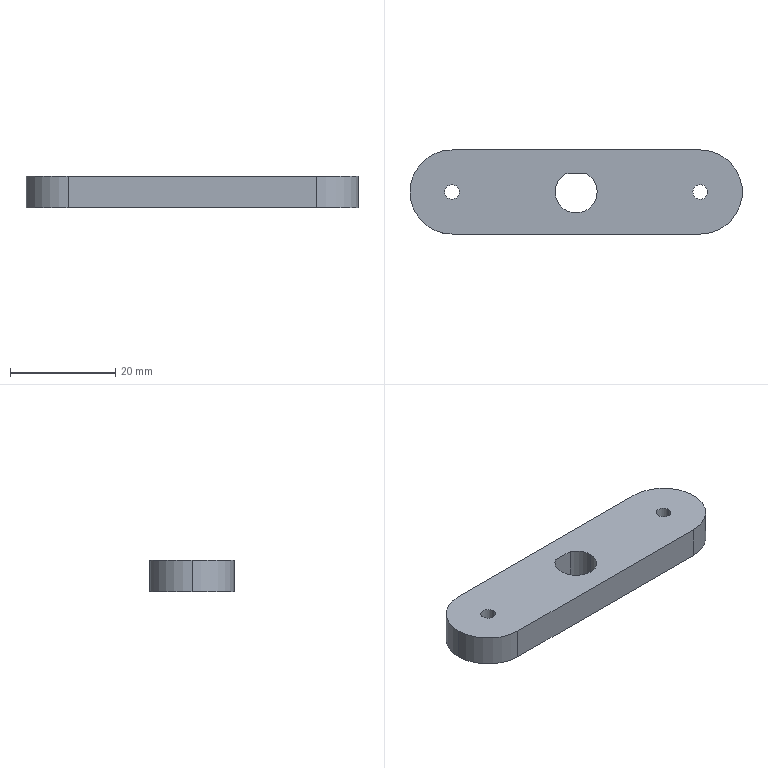Part | SolidWorks | features ICE 3, Extrusion 1 | 1 solid | 18 faces | box 63.2 x 16 x 6 mm | volume 5359 mm3 | cylinder 12 | plane 6 | commonest cylinder face diameters 2.8 x4 8 x3 16 x3 2 x2
STEP:
#1=CARTESIAN_POINT('',(-1.,4.5,3.));
#2=VERTEX_POINT('',#1);
#3=CARTESIAN_POINT('',(1.,4.5,3.));
#4=VERTEX_POINT('',#3);
#5=CARTESIAN_POINT('',(0.,4.5,3.));
#6=DIRECTION('',(0.,-1.,0.));
#7=DIRECTION('',(0.,0.,1.));
#8=AXIS2_PLACEMENT_3D('',#5,#6,#7);
#9=CIRCLE('',#8,1.);
#10=EDGE_CURVE('',#2,#4,#9,.T.);
#11=ORIENTED_EDGE('',*,*,#10,.T.);
#12=CARTESIAN_POINT('',(1.,8.,3.));
#13=VERTEX_POINT('',#12);
#14=CARTESIAN_POINT('',(1.,3.,3.));
#15=DIRECTION('',(0.,1.,0.));
#16=VECTOR('',#15,1000.);
#17=LINE('',#14,#16);
#18=EDGE_CURVE('',#4,#13,#17,.T.);
#19=ORIENTED_EDGE('',*,*,#18,.T.);
#20=CARTESIAN_POINT('',(-1.,8.,3.));
#21=VERTEX_POINT('',#20);
#22=CARTESIAN_POINT('',(0.,8.,3.));
#23=DIRECTION('',(0.,1.,0.));
#24=DIRECTION('',(-1.,0.,0.));
#25=AXIS2_PLACEMENT_3D('',#22,#23,#24);
#26=CIRCLE('',#25,1.);
#27=EDGE_CURVE('',#13,#21,#26,.T.);
#28=ORIENTED_EDGE('',*,*,#27,.T.);
#29=CARTESIAN_POINT('',(-1.,3.,3.));
#30=DIRECTION('',(0.,1.,0.));
#31=VECTOR('',#30,1000.);
#32=LINE('',#29,#31);
#33=EDGE_CURVE('',#2,#21,#32,.T.);
#34=ORIENTED_EDGE('',*,*,#33,.F.);
#35=EDGE_LOOP('',(#11,#19,#28,#34));
#36=FACE_OUTER_BOUND('',#35,.T.);
#37=CARTESIAN_POINT('',(0.,3.,3.));
#38=DIRECTION('',(0.,1.,0.));
#39=DIRECTION('',(-1.,0.,0.));
#40=AXIS2_PLACEMENT_3D('',#37,#38,#39);
#41=CYLINDRICAL_SURFACE('',#40,1.);
#42=ADVANCED_FACE('',(#36),#41,.F.);
#43=CARTESIAN_POINT('',(-25.,0.,0.));
#44=VERTEX_POINT('',#43);
#45=CARTESIAN_POINT('',(-22.2,0.,0.));
#46=VERTEX_POINT('',#45);
#47=CARTESIAN_POINT('',(-23.6,0.,0.));
#48=DIRECTION('',(0.,0.,1.));
#49=DIRECTION('',(1.,0.,0.));
#50=AXIS2_PLACEMENT_3D('',#47,#48,#49);
#51=CIRCLE('',#50,1.4);
#52=EDGE_CURVE('',#44,#46,#51,.T.);
#53=ORIENTED_EDGE('',*,*,#52,.F.);
#54=CARTESIAN_POINT('',(-25.,0.,6.));
#55=VERTEX_POINT('',#54);
#56=CARTESIAN_POINT('',(-25.,0.,0.));
#57=DIRECTION('',(0.,0.,1.));
#58=VECTOR('',#57,1000.);
#59=LINE('',#56,#58);
#60=EDGE_CURVE('',#44,#55,#59,.T.);
#61=ORIENTED_EDGE('',*,*,#60,.T.);
#62=CARTESIAN_POINT('',(-22.2,0.,6.));
#63=VERTEX_POINT('',#62);
#64=CARTESIAN_POINT('',(-23.6,0.,6.));
#65=DIRECTION('',(0.,0.,1.));
#66=DIRECTION('',(1.,0.,0.));
#67=AXIS2_PLACEMENT_3D('',#64,#65,#66);
#68=CIRCLE('',#67,1.4);
#69=EDGE_CURVE('',#55,#63,#68,.T.);
#70=ORIENTED_EDGE('',*,*,#69,.T.);
#71=CARTESIAN_POINT('',(-22.2,0.,0.));
#72=DIRECTION('',(0.,0.,1.));
#73=VECTOR('',#72,1000.);
#74=LINE('',#71,#73);
#75=EDGE_CURVE('',#46,#63,#74,.T.);
#76=ORIENTED_EDGE('',*,*,#75,.F.);
#77=EDGE_LOOP('',(#53,#61,#70,#76));
#78=FACE_OUTER_BOUND('',#77,.T.);
#79=CARTESIAN_POINT('',(-23.6,0.,0.));
#80=DIRECTION('',(0.,0.,1.));
#81=DIRECTION('',(1.,0.,0.));
#82=AXIS2_PLACEMENT_3D('',#79,#80,#81);
#83=CYLINDRICAL_SURFACE('',#82,1.4);
#84=ADVANCED_FACE('',(#78),#83,.F.);
#85=CARTESIAN_POINT('',(22.2,0.,0.));
#86=VERTEX_POINT('',#85);
#87=CARTESIAN_POINT('',(25.,0.,0.));
#88=VERTEX_POINT('',#87);
#89=CARTESIAN_POINT('',(23.6,0.,0.));
#90=DIRECTION('',(0.,0.,1.));
#91=DIRECTION('',(1.,0.,0.));
#92=AXIS2_PLACEMENT_3D('',#89,#90,#91);
#93=CIRCLE('',#92,1.4);
#94=EDGE_CURVE('',#86,#88,#93,.T.);
#95=ORIENTED_EDGE('',*,*,#94,.F.);
#96=CARTESIAN_POINT('',(22.2,0.,6.));
#97=VERTEX_POINT('',#96);
#98=CARTESIAN_POINT('',(22.2,0.,0.));
#99=DIRECTION('',(0.,0.,1.));
#100=VECTOR('',#99,1000.);
#101=LINE('',#98,#100);
#102=EDGE_CURVE('',#86,#97,#101,.T.);
#103=ORIENTED_EDGE('',*,*,#102,.T.);
#104=CARTESIAN_POINT('',(25.,0.,6.));
#105=VERTEX_POINT('',#104);
#106=CARTESIAN_POINT('',(23.6,0.,6.));
#107=DIRECTION('',(0.,0.,1.));
#108=DIRECTION('',(1.,0.,0.));
#109=AXIS2_PLACEMENT_3D('',#106,#107,#108);
#110=CIRCLE('',#109,1.4);
#111=EDGE_CURVE('',#97,#105,#110,.T.);
#112=ORIENTED_EDGE('',*,*,#111,.T.);
#113=CARTESIAN_POINT('',(25.,0.,0.));
#114=DIRECTION('',(0.,0.,1.));
#115=VECTOR('',#114,1000.);
#116=LINE('',#113,#115);
#117=EDGE_CURVE('',#88,#105,#116,.T.);
#118=ORIENTED_EDGE('',*,*,#117,.F.);
#119=EDGE_LOOP('',(#95,#103,#112,#118));
#120=FACE_OUTER_BOUND('',#119,.T.);
#121=CARTESIAN_POINT('',(23.6,0.,0.));
#122=DIRECTION('',(0.,0.,1.));
#123=DIRECTION('',(1.,0.,0.));
#124=AXIS2_PLACEMENT_3D('',#121,#122,#123);
#125=CYLINDRICAL_SURFACE('',#124,1.4);
#126=ADVANCED_FACE('',(#120),#125,.F.);
#127=CARTESIAN_POINT('',(-4.,0.,6.));
#128=VERTEX_POINT('',#127);
#129=CARTESIAN_POINT('',(4.,0.,6.));
#130=VERTEX_POINT('',#129);
#131=CARTESIAN_POINT('',(0.,0.,6.));
#132=DIRECTION('',(0.,0.,1.));
#133=DIRECTION('',(1.,0.,0.));
#134=AXIS2_PLACEMENT_3D('',#131,#132,#133);
#135=CIRCLE('',#134,4.);
#136=EDGE_CURVE('',#128,#130,#135,.T.);
#137=ORIENTED_EDGE('',*,*,#136,.T.);
#138=CARTESIAN_POINT('',(4.,0.,0.));
#139=VERTEX_POINT('',#138);
#140=CARTESIAN_POINT('',(4.,0.,6.));
#141=DIRECTION('',(0.,0.,-1.));
#142=VECTOR('',#141,1000.);
#143=LINE('',#140,#142);
#144=EDGE_CURVE('',#130,#139,#143,.T.);
#145=ORIENTED_EDGE('',*,*,#144,.T.);
#146=CARTESIAN_POINT('',(-4.,0.,0.));
#147=VERTEX_POINT('',#146);
#148=CARTESIAN_POINT('',(0.,0.,0.));
#149=DIRECTION('',(0.,0.,1.));
#150=DIRECTION('',(1.,0.,0.));
#151=AXIS2_PLACEMENT_3D('',#148,#149,#150);
#152=CIRCLE('',#151,4.);
#153=EDGE_CURVE('',#147,#139,#152,.T.);
#154=ORIENTED_EDGE('',*,*,#153,.F.);
#155=CARTESIAN_POINT('',(-4.,0.,6.));
#156=DIRECTION('',(0.,0.,-1.));
#157=VECTOR('',#156,1000.);
#158=LINE('',#155,#157);
#159=EDGE_CURVE('',#128,#147,#158,.T.);
#160=ORIENTED_EDGE('',*,*,#159,.F.);
#161=EDGE_LOOP('',(#137,#145,#154,#160));
#162=FACE_OUTER_BOUND('',#161,.T.);
#163=CARTESIAN_POINT('',(0.,0.,6.));
#164=DIRECTION('',(0.,0.,-1.));
#165=DIRECTION('',(-1.,0.,0.));
#166=AXIS2_PLACEMENT_3D('',#163,#164,#165);
#167=CYLINDRICAL_SURFACE('',#166,4.);
#168=ADVANCED_FACE('',(#162),#167,.F.);
#169=CARTESIAN_POINT('',(-1.936,3.5,6.));
#170=VERTEX_POINT('',#169);
#171=CARTESIAN_POINT('',(0.,0.,6.));
#172=DIRECTION('',(0.,0.,1.));
#173=DIRECTION('',(1.,0.,0.));
#174=AXIS2_PLACEMENT_3D('',#171,#172,#173);
#175=CIRCLE('',#174,4.);
#176=EDGE_CURVE('',#170,#128,#175,.T.);
#177=ORIENTED_EDGE('',*,*,#176,.T.);
#178=ORIENTED_EDGE('',*,*,#159,.T.);
#179=CARTESIAN_POINT('',(-1.936,3.5,0.));
#180=VERTEX_POINT('',#179);
#181=CARTESIAN_POINT('',(0.,0.,0.));
#182=DIRECTION('',(0.,0.,1.));
#183=DIRECTION('',(1.,0.,0.));
#184=AXIS2_PLACEMENT_3D('',#181,#182,#183);
#185=CIRCLE('',#184,4.);
#186=EDGE_CURVE('',#180,#147,#185,.T.);
#187=ORIENTED_EDGE('',*,*,#186,.F.);
#188=CARTESIAN_POINT('',(-1.936,3.5,6.));
#189=DIRECTION('',(0.,0.,-1.));
#190=VECTOR('',#189,1000.);
#191=LINE('',#188,#190);
#192=EDGE_CURVE('',#170,#180,#191,.T.);
#193=ORIENTED_EDGE('',*,*,#192,.F.);
#194=EDGE_LOOP('',(#177,#178,#187,#193));
#195=FACE_OUTER_BOUND('',#194,.T.);
#196=CARTESIAN_POINT('',(0.,0.,6.));
#197=DIRECTION('',(0.,0.,-1.));
#198=DIRECTION('',(-1.,0.,0.));
#199=AXIS2_PLACEMENT_3D('',#196,#197,#198);
#200=CYLINDRICAL_SURFACE('',#199,4.);
#201=ADVANCED_FACE('',(#195),#200,.F.);
#202=CARTESIAN_POINT('',(-31.6,0.,6.));
#203=VERTEX_POINT('',#202);
#204=CARTESIAN_POINT('',(-23.6,-8.,6.));
#205=VERTEX_POINT('',#204);
#206=CARTESIAN_POINT('',(-23.6,0.,6.));
#207=DIRECTION('',(0.,0.,1.));
#208=DIRECTION('',(1.,0.,0.));
#209=AXIS2_PLACEMENT_3D('',#206,#207,#208);
#210=CIRCLE('',#209,8.);
#211=EDGE_CURVE('',#203,#205,#210,.T.);
#212=ORIENTED_EDGE('',*,*,#211,.F.);
#213=CARTESIAN_POINT('',(-31.6,0.,0.));
#214=VERTEX_POINT('',#213);
#215=CARTESIAN_POINT('',(-31.6,0.,6.));
#216=DIRECTION('',(0.,0.,-1.));
#217=VECTOR('',#216,1000.);
#218=LINE('',#215,#217);
#219=EDGE_CURVE('',#203,#214,#218,.T.);
#220=ORIENTED_EDGE('',*,*,#219,.T.);
#221=CARTESIAN_POINT('',(-23.6,-8.,0.));
#222=VERTEX_POINT('',#221);
#223=CARTESIAN_POINT('',(-23.6,0.,0.));
#224=DIRECTION('',(0.,0.,1.));
#225=DIRECTION('',(1.,0.,0.));
#226=AXIS2_PLACEMENT_3D('',#223,#224,#225);
#227=CIRCLE('',#226,8.);
#228=EDGE_CURVE('',#214,#222,#227,.T.);
#229=ORIENTED_EDGE('',*,*,#228,.T.);
#230=CARTESIAN_POINT('',(-23.6,-8.,6.));
#231=DIRECTION('',(0.,0.,-1.));
#232=VECTOR('',#231,1000.);
#233=LINE('',#230,#232);
#234=EDGE_CURVE('',#205,#222,#233,.T.);
#235=ORIENTED_EDGE('',*,*,#234,.F.);
#236=EDGE_LOOP('',(#212,#220,#229,#235));
#237=FACE_OUTER_BOUND('',#236,.T.);
#238=CARTESIAN_POINT('',(-23.6,0.,6.));
#239=DIRECTION('',(0.,0.,-1.));
#240=DIRECTION('',(-1.,0.,0.));
#241=AXIS2_PLACEMENT_3D('',#238,#239,#240);
#242=CYLINDRICAL_SURFACE('',#241,8.);
#243=ADVANCED_FACE('',(#237),#242,.T.);
#244=ORIENTED_EDGE('',*,*,#176,.F.);
#245=CARTESIAN_POINT('',(1.936,3.5,6.));
#246=VERTEX_POINT('',#245);
#247=CARTESIAN_POINT('',(2.48,3.5,6.));
#248=DIRECTION('',(-1.,0.,0.));
#249=VECTOR('',#248,1000.);
#250=LINE('',#247,#249);
#251=EDGE_CURVE('',#246,#170,#250,.T.);
#252=ORIENTED_EDGE('',*,*,#251,.F.);
#253=CARTESIAN_POINT('',(0.,0.,6.));
#254=DIRECTION('',(0.,0.,1.));
#255=DIRECTION('',(1.,0.,0.));
#256=AXIS2_PLACEMENT_3D('',#253,#254,#255);
#257=CIRCLE('',#256,4.);
#258=EDGE_CURVE('',#130,#246,#257,.T.);
#259=ORIENTED_EDGE('',*,*,#258,.F.);
#260=ORIENTED_EDGE('',*,*,#136,.F.);
#261=EDGE_LOOP('',(#244,#252,#259,#260));
#262=FACE_BOUND('',#261,.T.);
#263=CARTESIAN_POINT('',(-23.6,0.,6.));
#264=DIRECTION('',(0.,0.,1.));
#265=DIRECTION('',(1.,0.,0.));
#266=AXIS2_PLACEMENT_3D('',#263,#264,#265);
#267=CIRCLE('',#266,1.4);
#268=EDGE_CURVE('',#63,#55,#267,.T.);
#269=ORIENTED_EDGE('',*,*,#268,.F.);
#270=ORIENTED_EDGE('',*,*,#69,.F.);
#271=EDGE_LOOP('',(#269,#270));
#272=FACE_BOUND('',#271,.T.);
#273=CARTESIAN_POINT('',(23.6,0.,6.));
#274=DIRECTION('',(0.,0.,1.));
#275=DIRECTION('',(1.,0.,0.));
#276=AXIS2_PLACEMENT_3D('',#273,#274,#275);
#277=CIRCLE('',#276,1.4);
#278=EDGE_CURVE('',#105,#97,#277,.T.);
#279=ORIENTED_EDGE('',*,*,#278,.F.);
#280=ORIENTED_EDGE('',*,*,#111,.F.);
#281=EDGE_LOOP('',(#279,#280));
#282=FACE_BOUND('',#281,.T.);
#283=CARTESIAN_POINT('',(-23.6,8.,6.));
#284=VERTEX_POINT('',#283);
#285=CARTESIAN_POINT('',(-23.6,0.,6.));
#286=DIRECTION('',(0.,0.,1.));
#287=DIRECTION('',(1.,0.,0.));
#288=AXIS2_PLACEMENT_3D('',#285,#286,#287);
#289=CIRCLE('',#288,8.);
#290=EDGE_CURVE('',#284,#203,#289,.T.);
#291=ORIENTED_EDGE('',*,*,#290,.T.);
#292=ORIENTED_EDGE('',*,*,#211,.T.);
#293=CARTESIAN_POINT('',(23.6,-8.,6.));
#294=VERTEX_POINT('',#293);
#295=CARTESIAN_POINT('',(-23.6,-8.,6.));
#296=DIRECTION('',(1.,0.,0.));
#297=VECTOR('',#296,1000.);
#298=LINE('',#295,#297);
#299=EDGE_CURVE('',#205,#294,#298,.T.);
#300=ORIENTED_EDGE('',*,*,#299,.T.);
#301=CARTESIAN_POINT('',(23.6,8.,6.));
#302=VERTEX_POINT('',#301);
#303=CARTESIAN_POINT('',(23.6,0.,6.));
#304=DIRECTION('',(0.,0.,1.));
#305=DIRECTION('',(1.,0.,0.));
#306=AXIS2_PLACEMENT_3D('',#303,#304,#305);
#307=CIRCLE('',#306,8.);
#308=EDGE_CURVE('',#294,#302,#307,.T.);
#309=ORIENTED_EDGE('',*,*,#308,.T.);
#310=CARTESIAN_POINT('',(-23.6,8.,6.));
#311=DIRECTION('',(-1.,0.,0.));
#312=VECTOR('',#311,1000.);
#313=LINE('',#310,#312);
#314=EDGE_CURVE('',#302,#284,#313,.T.);
#315=ORIENTED_EDGE('',*,*,#314,.T.);
#316=EDGE_LOOP('',(#291,#292,#300,#309,#315));
#317=FACE_OUTER_BOUND('',#316,.T.);
#318=CARTESIAN_POINT('',(-23.6,0.,6.));
#319=DIRECTION('',(0.,0.,1.));
#320=DIRECTION('',(1.,0.,0.));
#321=AXIS2_PLACEMENT_3D('',#318,#319,#320);
#322=PLANE('',#321);
#323=ADVANCED_FACE('',(#262,#272,#282,#317),#322,.T.);
#324=CARTESIAN_POINT('',(1.936,3.5,0.));
#325=VERTEX_POINT('',#324);
#326=CARTESIAN_POINT('',(2.48,3.5,0.));
#327=DIRECTION('',(-1.,0.,0.));
#328=VECTOR('',#327,1000.);
#329=LINE('',#326,#328);
#330=EDGE_CURVE('',#325,#180,#329,.T.);
#331=ORIENTED_EDGE('',*,*,#330,.T.);
#332=ORIENTED_EDGE('',*,*,#186,.T.);
#333=ORIENTED_EDGE('',*,*,#153,.T.);
#334=CARTESIAN_POINT('',(0.,0.,0.));
#335=DIRECTION('',(0.,0.,1.));
#336=DIRECTION('',(1.,0.,0.));
#337=AXIS2_PLACEMENT_3D('',#334,#335,#336);
#338=CIRCLE('',#337,4.);
#339=EDGE_CURVE('',#139,#325,#338,.T.);
#340=ORIENTED_EDGE('',*,*,#339,.T.);
#341=EDGE_LOOP('',(#331,#332,#333,#340));
#342=FACE_BOUND('',#341,.T.);
#343=CARTESIAN_POINT('',(-23.6,0.,0.));
#344=DIRECTION('',(0.,0.,1.));
#345=DIRECTION('',(1.,0.,0.));
#346=AXIS2_PLACEMENT_3D('',#343,#344,#345);
#347=CIRCLE('',#346,1.4);
#348=EDGE_CURVE('',#46,#44,#347,.T.);
#349=ORIENTED_EDGE('',*,*,#348,.T.);
#350=ORIENTED_EDGE('',*,*,#52,.T.);
#351=EDGE_LOOP('',(#349,#350));
#352=FACE_BOUND('',#351,.T.);
#353=CARTESIAN_POINT('',(23.6,0.,0.));
#354=DIRECTION('',(0.,0.,1.));
#355=DIRECTION('',(1.,0.,0.));
#356=AXIS2_PLACEMENT_3D('',#353,#354,#355);
#357=CIRCLE('',#356,1.4);
#358=EDGE_CURVE('',#88,#86,#357,.T.);
#359=ORIENTED_EDGE('',*,*,#358,.T.);
#360=ORIENTED_EDGE('',*,*,#94,.T.);
#361=EDGE_LOOP('',(#359,#360));
#362=FACE_BOUND('',#361,.T.);
#363=CARTESIAN_POINT('',(-23.6,8.,0.));
#364=VERTEX_POINT('',#363);
#365=CARTESIAN_POINT('',(-23.6,0.,0.));
#366=DIRECTION('',(0.,0.,1.));
#367=DIRECTION('',(1.,0.,0.));
#368=AXIS2_PLACEMENT_3D('',#365,#366,#367);
#369=CIRCLE('',#368,8.);
#370=EDGE_CURVE('',#364,#214,#369,.T.);
#371=ORIENTED_EDGE('',*,*,#370,.F.);
#372=CARTESIAN_POINT('',(23.6,8.,0.));
#373=VERTEX_POINT('',#372);
#374=CARTESIAN_POINT('',(-23.6,8.,0.));
#375=DIRECTION('',(-1.,0.,0.));
#376=VECTOR('',#375,1000.);
#377=LINE('',#374,#376);
#378=EDGE_CURVE('',#373,#364,#377,.T.);
#379=ORIENTED_EDGE('',*,*,#378,.F.);
#380=CARTESIAN_POINT('',(23.6,-8.,0.));
#381=VERTEX_POINT('',#380);
#382=CARTESIAN_POINT('',(23.6,0.,0.));
#383=DIRECTION('',(0.,0.,1.));
#384=DIRECTION('',(1.,0.,0.));
#385=AXIS2_PLACEMENT_3D('',#382,#383,#384);
#386=CIRCLE('',#385,8.);
#387=EDGE_CURVE('',#381,#373,#386,.T.);
#388=ORIENTED_EDGE('',*,*,#387,.F.);
#389=CARTESIAN_POINT('',(-23.6,-8.,0.));
#390=DIRECTION('',(1.,0.,0.));
#391=VECTOR('',#390,1000.);
#392=LINE('',#389,#391);
#393=EDGE_CURVE('',#222,#381,#392,.T.);
#394=ORIENTED_EDGE('',*,*,#393,.F.);
#395=ORIENTED_EDGE('',*,*,#228,.F.);
#396=EDGE_LOOP('',(#371,#379,#388,#394,#395));
#397=FACE_OUTER_BOUND('',#396,.T.);
#398=CARTESIAN_POINT('',(-23.6,0.,0.));
#399=DIRECTION('',(0.,0.,1.));
#400=DIRECTION('',(1.,0.,0.));
#401=AXIS2_PLACEMENT_3D('',#398,#399,#400);
#402=PLANE('',#401);
#403=ADVANCED_FACE('',(#342,#352,#362,#397),#402,.F.);
#404=ORIENTED_EDGE('',*,*,#219,.F.);
#405=ORIENTED_EDGE('',*,*,#290,.F.);
#406=CARTESIAN_POINT('',(-23.6,8.,6.));
#407=DIRECTION('',(0.,0.,-1.));
#408=VECTOR('',#407,1000.);
#409=LINE('',#406,#408);
#410=EDGE_CURVE('',#284,#364,#409,.T.);
#411=ORIENTED_EDGE('',*,*,#410,.T.);
#412=ORIENTED_EDGE('',*,*,#370,.T.);
#413=EDGE_LOOP('',(#404,#405,#411,#412));
#414=FACE_OUTER_BOUND('',#413,.T.);
#415=CARTESIAN_POINT('',(-23.6,0.,6.));
#416=DIRECTION('',(0.,0.,-1.));
#417=DIRECTION('',(-1.,0.,0.));
#418=AXIS2_PLACEMENT_3D('',#415,#416,#417);
#419=CYLINDRICAL_SURFACE('',#418,8.);
#420=ADVANCED_FACE('',(#414),#419,.T.);
#421=ORIENTED_EDGE('',*,*,#393,.T.);
#422=CARTESIAN_POINT('',(23.6,-8.,6.));
#423=DIRECTION('',(0.,0.,-1.));
#424=VECTOR('',#423,1000.);
#425=LINE('',#422,#424);
#426=EDGE_CURVE('',#294,#381,#425,.T.);
#427=ORIENTED_EDGE('',*,*,#426,.F.);
#428=ORIENTED_EDGE('',*,*,#299,.F.);
#429=ORIENTED_EDGE('',*,*,#234,.T.);
#430=EDGE_LOOP('',(#421,#427,#428,#429));
#431=FACE_OUTER_BOUND('',#430,.T.);
#432=CARTESIAN_POINT('',(-23.6,-8.,6.));
#433=DIRECTION('',(0.,1.,0.));
#434=DIRECTION('',(-1.,0.,0.));
#435=AXIS2_PLACEMENT_3D('',#432,#433,#434);
#436=PLANE('',#435);
#437=ADVANCED_FACE('',(#431),#436,.F.);
#438=ORIENTED_EDGE('',*,*,#387,.T.);
#439=CARTESIAN_POINT('',(23.6,8.,6.));
#440=DIRECTION('',(0.,0.,-1.));
#441=VECTOR('',#440,1000.);
#442=LINE('',#439,#441);
#443=EDGE_CURVE('',#302,#373,#442,.T.);
#444=ORIENTED_EDGE('',*,*,#443,.F.);
#445=ORIENTED_EDGE('',*,*,#308,.F.);
#446=ORIENTED_EDGE('',*,*,#426,.T.);
#447=EDGE_LOOP('',(#438,#444,#445,#446));
#448=FACE_OUTER_BOUND('',#447,.T.);
#449=CARTESIAN_POINT('',(23.6,0.,6.));
#450=DIRECTION('',(0.,0.,-1.));
#451=DIRECTION('',(-1.,0.,0.));
#452=AXIS2_PLACEMENT_3D('',#449,#450,#451);
#453=CYLINDRICAL_SURFACE('',#452,8.);
#454=ADVANCED_FACE('',(#448),#453,.T.);
#455=CARTESIAN_POINT('',(0.,8.,3.));
#456=DIRECTION('',(0.,1.,0.));
#457=DIRECTION('',(-1.,0.,0.));
#458=AXIS2_PLACEMENT_3D('',#455,#456,#457);
#459=CIRCLE('',#458,1.);
#460=EDGE_CURVE('',#21,#13,#459,.T.);
#461=ORIENTED_EDGE('',*,*,#460,.F.);
#462=ORIENTED_EDGE('',*,*,#27,.F.);
#463=EDGE_LOOP('',(#461,#462));
#464=FACE_BOUND('',#463,.T.);
#465=ORIENTED_EDGE('',*,*,#378,.T.);
#466=ORIENTED_EDGE('',*,*,#410,.F.);
#467=ORIENTED_EDGE('',*,*,#314,.F.);
#468=ORIENTED_EDGE('',*,*,#443,.T.);
#469=EDGE_LOOP('',(#465,#466,#467,#468));
#470=FACE_OUTER_BOUND('',#469,.T.);
#471=CARTESIAN_POINT('',(-23.6,8.,6.));
#472=DIRECTION('',(0.,-1.,0.));
#473=DIRECTION('',(1.,0.,0.));
#474=AXIS2_PLACEMENT_3D('',#471,#472,#473);
#475=PLANE('',#474);
#476=ADVANCED_FACE('',(#464,#470),#475,.F.);
#477=ORIENTED_EDGE('',*,*,#144,.F.);
#478=ORIENTED_EDGE('',*,*,#258,.T.);
#479=CARTESIAN_POINT('',(1.936,3.5,6.));
#480=DIRECTION('',(0.,0.,1.));
#481=VECTOR('',#480,1000.);
#482=LINE('',#479,#481);
#483=EDGE_CURVE('',#325,#246,#482,.T.);
#484=ORIENTED_EDGE('',*,*,#483,.F.);
#485=ORIENTED_EDGE('',*,*,#339,.F.);
#486=EDGE_LOOP('',(#477,#478,#484,#485));
#487=FACE_OUTER_BOUND('',#486,.T.);
#488=CARTESIAN_POINT('',(0.,0.,6.));
#489=DIRECTION('',(0.,0.,-1.));
#490=DIRECTION('',(-1.,0.,0.));
#491=AXIS2_PLACEMENT_3D('',#488,#489,#490);
#492=CYLINDRICAL_SURFACE('',#491,4.);
#493=ADVANCED_FACE('',(#487),#492,.F.);
#494=ORIENTED_EDGE('',*,*,#102,.F.);
#495=ORIENTED_EDGE('',*,*,#358,.F.);
#496=ORIENTED_EDGE('',*,*,#117,.T.);
#497=ORIENTED_EDGE('',*,*,#278,.T.);
#498=EDGE_LOOP('',(#494,#495,#496,#497));
#499=FACE_OUTER_BOUND('',#498,.T.);
#500=CARTESIAN_POINT('',(23.6,0.,0.));
#501=DIRECTION('',(0.,0.,1.));
#502=DIRECTION('',(1.,0.,0.));
#503=AXIS2_PLACEMENT_3D('',#500,#501,#502);
#504=CYLINDRICAL_SURFACE('',#503,1.4);
#505=ADVANCED_FACE('',(#499),#504,.F.);
#506=ORIENTED_EDGE('',*,*,#60,.F.);
#507=ORIENTED_EDGE('',*,*,#348,.F.);
#508=ORIENTED_EDGE('',*,*,#75,.T.);
#509=ORIENTED_EDGE('',*,*,#268,.T.);
#510=EDGE_LOOP('',(#506,#507,#508,#509));
#511=FACE_OUTER_BOUND('',#510,.T.);
#512=CARTESIAN_POINT('',(-23.6,0.,0.));
#513=DIRECTION('',(0.,0.,1.));
#514=DIRECTION('',(1.,0.,0.));
#515=AXIS2_PLACEMENT_3D('',#512,#513,#514);
#516=CYLINDRICAL_SURFACE('',#515,1.4);
#517=ADVANCED_FACE('',(#511),#516,.F.);
#518=ORIENTED_EDGE('',*,*,#18,.F.);
#519=CARTESIAN_POINT('',(0.,4.5,3.));
#520=DIRECTION('',(0.,-1.,0.));
#521=DIRECTION('',(0.,0.,1.));
#522=AXIS2_PLACEMENT_3D('',#519,#520,#521);
#523=CIRCLE('',#522,1.);
#524=EDGE_CURVE('',#4,#2,#523,.T.);
#525=ORIENTED_EDGE('',*,*,#524,.T.);
#526=ORIENTED_EDGE('',*,*,#33,.T.);
#527=ORIENTED_EDGE('',*,*,#460,.T.);
#528=EDGE_LOOP('',(#518,#525,#526,#527));
#529=FACE_OUTER_BOUND('',#528,.T.);
#530=CARTESIAN_POINT('',(0.,3.,3.));
#531=DIRECTION('',(0.,1.,0.));
#532=DIRECTION('',(-1.,0.,0.));
#533=AXIS2_PLACEMENT_3D('',#530,#531,#532);
#534=CYLINDRICAL_SURFACE('',#533,1.);
#535=ADVANCED_FACE('',(#529),#534,.F.);
#536=ORIENTED_EDGE('',*,*,#10,.F.);
#537=ORIENTED_EDGE('',*,*,#524,.F.);
#538=EDGE_LOOP('',(#536,#537));
#539=FACE_OUTER_BOUND('',#538,.T.);
#540=CARTESIAN_POINT('',(2.48,4.5,11.06));
#541=DIRECTION('',(0.,1.,0.));
#542=DIRECTION('',(0.,0.,1.));
#543=AXIS2_PLACEMENT_3D('',#540,#541,#542);
#544=PLANE('',#543);
#545=ADVANCED_FACE('',(#539),#544,.T.);
#546=ORIENTED_EDGE('',*,*,#251,.T.);
#547=ORIENTED_EDGE('',*,*,#192,.T.);
#548=ORIENTED_EDGE('',*,*,#330,.F.);
#549=ORIENTED_EDGE('',*,*,#483,.T.);
#550=EDGE_LOOP('',(#546,#547,#548,#549));
#551=FACE_OUTER_BOUND('',#550,.T.);
#552=CARTESIAN_POINT('',(2.48,3.5,11.06));
#553=DIRECTION('',(0.,-1.,0.));
#554=DIRECTION('',(0.,0.,-1.));
#555=AXIS2_PLACEMENT_3D('',#552,#553,#554);
#556=PLANE('',#555);
#557=ADVANCED_FACE('',(#551),#556,.T.);
#558=CLOSED_SHELL('',(#42,#84,#126,#168,#201,#243,#323,#403,#420,#437,#454,#476,#493,#505,#517,#535,#545,#557));
#559=MANIFOLD_SOLID_BREP('',#558);
#560=CARTESIAN_POINT('',(0.,0.,0.));
#561=DIRECTION('',(0.,0.,1.));
#562=DIRECTION('',(1.,0.,0.));
#563=AXIS2_PLACEMENT_3D('',#560,#561,#562);
#564=(LENGTH_UNIT()NAMED_UNIT(*)SI_UNIT(.MILLI.,.METRE.));
#565=UNCERTAINTY_MEASURE_WITH_UNIT(LENGTH_MEASURE(0.00001),#564,'','');
#566=(NAMED_UNIT(*)PLANE_ANGLE_UNIT()SI_UNIT($,.RADIAN.));
#567=(NAMED_UNIT(*)SI_UNIT($,.STERADIAN.)SOLID_ANGLE_UNIT());
#568=(GEOMETRIC_REPRESENTATION_CONTEXT(3)GLOBAL_UNCERTAINTY_ASSIGNED_CONTEXT((#565))GLOBAL_UNIT_ASSIGNED_CONTEXT((#564,#566,#567))REPRESENTATION_CONTEXT('',''));
#569=ADVANCED_BREP_SHAPE_REPRESENTATION('',(#559,#563),#568);